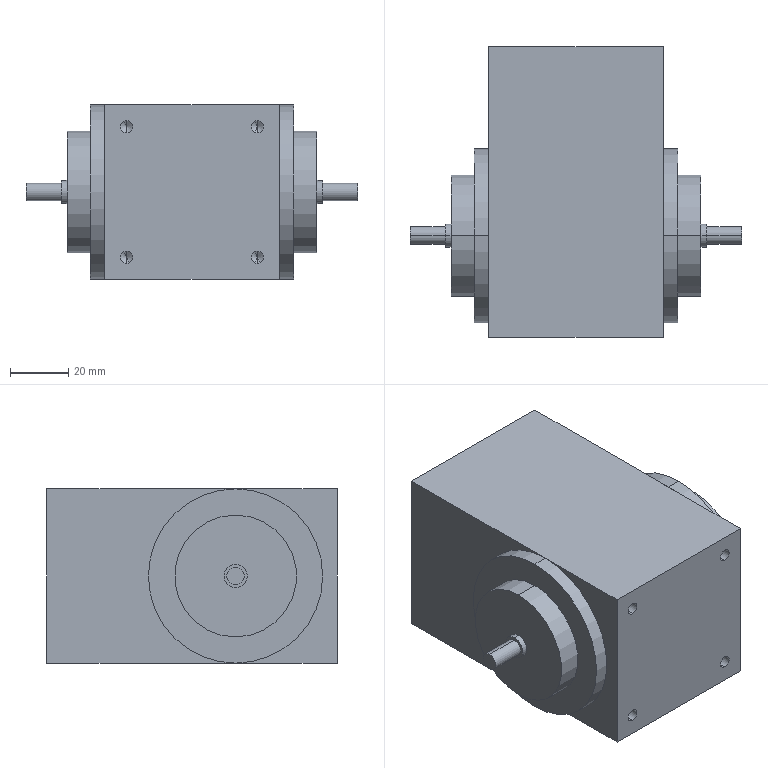Part | STEP file | PN_0007TM301_Default | 1 solid | 48 faces | box 114 x 100 x 60 mm | volume 410522 mm3 | cylinder 24 | plane 16 | cone 8 | commonest cylinder face diameters 4.2 x8 6 x4 8 x4 42 x4 60 x4